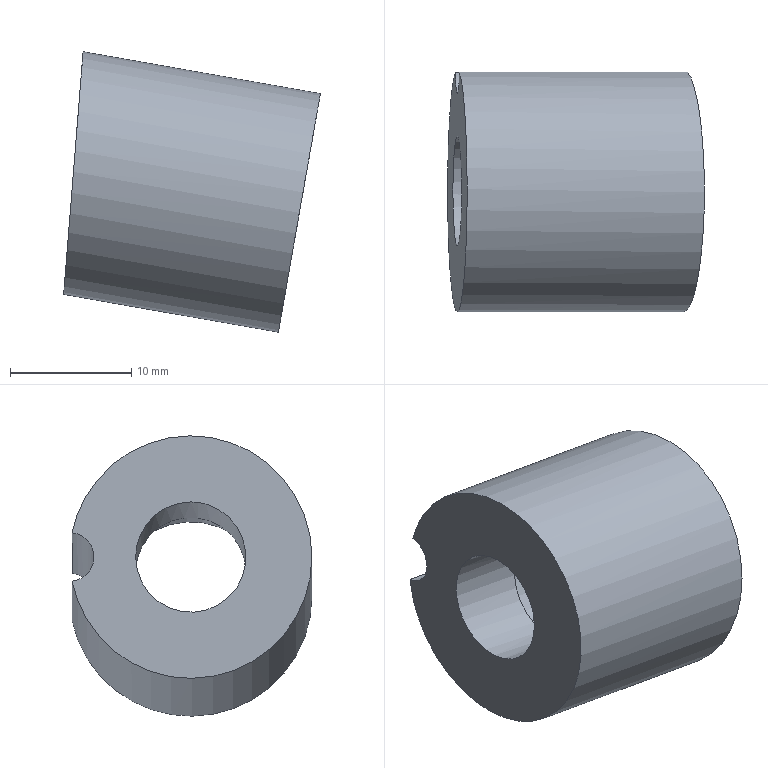Part | NX | features solid 2 | 1 solid | 7 faces | box 21.197 x 19.8 x 23.15 mm | volume 3890 mm3 | cylinder 4 | plane 3 | commonest cylinder face diameters 4 x1 9.1 x1 12.6 x1 20 x1
STEP:
#1=CARTESIAN_POINT('',(-453.088,686.016,-36.598));
#2=VERTEX_POINT('',#1);
#3=CARTESIAN_POINT('',(-434.245,686.016,-39.921));
#4=VERTEX_POINT('',#3);
#5=CARTESIAN_POINT('',(-444.093,686.016,-38.184));
#6=DIRECTION('',(-0.9848,0.,0.1736));
#7=VECTOR('',#6,1000.);
#8=LINE('',#5,#7);
#9=EDGE_CURVE('',#2,#4,#8,.F.);
#10=ORIENTED_EDGE('',*,*,#9,.F.);
#11=CARTESIAN_POINT('',(-453.408,686.016,-40.583));
#12=VERTEX_POINT('',#11);
#13=CARTESIAN_POINT('',(-453.248,676.216,-38.591));
#14=DIRECTION('',(-0.9968,0.,0.08003));
#15=DIRECTION('',(0.08003,0.,0.9968));
#16=AXIS2_PLACEMENT_3D('',#13,#14,#15);
#17=ELLIPSE('',#16,10.045,10.);
#18=EDGE_CURVE('',#2,#12,#17,.F.);
#19=ORIENTED_EDGE('',*,*,#18,.T.);
#20=CARTESIAN_POINT('',(-434.936,686.016,-43.84));
#21=VERTEX_POINT('',#20);
#22=CARTESIAN_POINT('',(-444.784,686.016,-42.104));
#23=DIRECTION('',(-0.9848,0.,0.1736));
#24=VECTOR('',#23,1000.);
#25=LINE('',#22,#24);
#26=EDGE_CURVE('',#21,#12,#25,.T.);
#27=ORIENTED_EDGE('',*,*,#26,.F.);
#28=CARTESIAN_POINT('',(-434.591,676.216,-41.881));
#29=DIRECTION('',(-0.9848,0.,0.1736));
#30=DIRECTION('',(0.,1.,0.));
#31=AXIS2_PLACEMENT_3D('',#28,#29,#30);
#32=CIRCLE('',#31,10.);
#33=EDGE_CURVE('',#21,#4,#32,.T.);
#34=ORIENTED_EDGE('',*,*,#33,.T.);
#35=EDGE_LOOP('',(#10,#19,#27,#34));
#36=FACE_BOUND('',#35,.T.);
#37=CARTESIAN_POINT('',(-434.591,676.216,-41.881));
#38=DIRECTION('',(-0.9848,0.,0.1736));
#39=DIRECTION('',(0.,1.,0.));
#40=AXIS2_PLACEMENT_3D('',#37,#38,#39);
#41=CYLINDRICAL_SURFACE('',#40,10.);
#42=ADVANCED_FACE('',(#36),#41,.T.);
#43=CARTESIAN_POINT('',(-453.248,686.216,-38.591));
#44=DIRECTION('',(-0.9968,0.,0.08003));
#45=DIRECTION('',(0.08003,0.,0.9968));
#46=AXIS2_PLACEMENT_3D('',#43,#44,#45);
#47=ELLIPSE('',#46,2.009,2.);
#48=EDGE_CURVE('',#2,#12,#47,.F.);
#49=ORIENTED_EDGE('',*,*,#48,.F.);
#50=ORIENTED_EDGE('',*,*,#9,.T.);
#51=CARTESIAN_POINT('',(-434.591,686.216,-41.881));
#52=DIRECTION('',(-0.9848,0.,0.1736));
#53=DIRECTION('',(0.,1.,0.));
#54=AXIS2_PLACEMENT_3D('',#51,#52,#53);
#55=CIRCLE('',#54,2.);
#56=EDGE_CURVE('',#21,#4,#55,.T.);
#57=ORIENTED_EDGE('',*,*,#56,.F.);
#58=ORIENTED_EDGE('',*,*,#26,.T.);
#59=EDGE_LOOP('',(#49,#50,#57,#58));
#60=FACE_BOUND('',#59,.T.);
#61=CARTESIAN_POINT('',(-434.591,686.216,-41.881));
#62=DIRECTION('',(-0.9848,0.,0.1736));
#63=DIRECTION('',(0.,1.,0.));
#64=AXIS2_PLACEMENT_3D('',#61,#62,#63);
#65=CYLINDRICAL_SURFACE('',#64,2.);
#66=ADVANCED_FACE('',(#60),#65,.F.);
#67=CARTESIAN_POINT('',(-446.408,680.766,-39.797));
#68=VERTEX_POINT('',#67);
#69=CARTESIAN_POINT('',(-446.408,676.216,-39.797));
#70=DIRECTION('',(-0.9848,0.,0.1736));
#71=DIRECTION('',(0.,1.,0.));
#72=AXIS2_PLACEMENT_3D('',#69,#70,#71);
#73=CIRCLE('',#72,4.55);
#74=EDGE_CURVE('',#68,#68,#73,.T.);
#75=ORIENTED_EDGE('',*,*,#74,.F.);
#76=EDGE_LOOP('',(#75));
#77=FACE_BOUND('',#76,.T.);
#78=CARTESIAN_POINT('',(-452.882,676.216,-34.035));
#79=VERTEX_POINT('',#78);
#80=CARTESIAN_POINT('',(-453.248,676.216,-38.591));
#81=DIRECTION('',(-0.9968,0.,0.08003));
#82=DIRECTION('',(0.08003,0.,0.9968));
#83=AXIS2_PLACEMENT_3D('',#80,#81,#82);
#84=ELLIPSE('',#83,4.57,4.55);
#85=EDGE_CURVE('',#79,#79,#84,.F.);
#86=ORIENTED_EDGE('',*,*,#85,.F.);
#87=EDGE_LOOP('',(#86));
#88=FACE_BOUND('',#87,.T.);
#89=CARTESIAN_POINT('',(-434.591,676.216,-41.881));
#90=DIRECTION('',(-0.9848,0.,0.1736));
#91=DIRECTION('',(0.,1.,0.));
#92=AXIS2_PLACEMENT_3D('',#89,#90,#91);
#93=CYLINDRICAL_SURFACE('',#92,4.55);
#94=ADVANCED_FACE('',(#77,#88),#93,.F.);
#95=CARTESIAN_POINT('',(-434.591,682.516,-41.881));
#96=VERTEX_POINT('',#95);
#97=CARTESIAN_POINT('',(-434.591,676.216,-41.881));
#98=DIRECTION('',(-0.9848,0.,0.1736));
#99=DIRECTION('',(0.,1.,0.));
#100=AXIS2_PLACEMENT_3D('',#97,#98,#99);
#101=CIRCLE('',#100,6.3);
#102=EDGE_CURVE('',#96,#96,#101,.T.);
#103=ORIENTED_EDGE('',*,*,#102,.T.);
#104=EDGE_LOOP('',(#103));
#105=FACE_BOUND('',#104,.T.);
#106=ORIENTED_EDGE('',*,*,#33,.F.);
#107=ORIENTED_EDGE('',*,*,#56,.T.);
#108=EDGE_LOOP('',(#106,#107));
#109=FACE_BOUND('',#108,.T.);
#110=CARTESIAN_POINT('',(-434.591,676.216,-41.881));
#111=DIRECTION('',(-0.9848,0.,0.1736));
#112=DIRECTION('',(0.,1.,0.));
#113=AXIS2_PLACEMENT_3D('',#110,#111,#112);
#114=PLANE('',#113);
#115=ADVANCED_FACE('',(#105,#109),#114,.F.);
#116=ORIENTED_EDGE('',*,*,#102,.F.);
#117=EDGE_LOOP('',(#116));
#118=FACE_BOUND('',#117,.T.);
#119=CARTESIAN_POINT('',(-446.408,682.516,-39.797));
#120=VERTEX_POINT('',#119);
#121=CARTESIAN_POINT('',(-446.408,676.216,-39.797));
#122=DIRECTION('',(-0.9848,0.,0.1736));
#123=DIRECTION('',(0.,1.,0.));
#124=AXIS2_PLACEMENT_3D('',#121,#122,#123);
#125=CIRCLE('',#124,6.3);
#126=EDGE_CURVE('',#120,#120,#125,.T.);
#127=ORIENTED_EDGE('',*,*,#126,.T.);
#128=EDGE_LOOP('',(#127));
#129=FACE_BOUND('',#128,.T.);
#130=CARTESIAN_POINT('',(-434.591,676.216,-41.881));
#131=DIRECTION('',(-0.9848,0.,0.1736));
#132=DIRECTION('',(0.,1.,0.));
#133=AXIS2_PLACEMENT_3D('',#130,#131,#132);
#134=CYLINDRICAL_SURFACE('',#133,6.3);
#135=ADVANCED_FACE('',(#118,#129),#134,.F.);
#136=ORIENTED_EDGE('',*,*,#74,.T.);
#137=EDGE_LOOP('',(#136));
#138=FACE_BOUND('',#137,.T.);
#139=ORIENTED_EDGE('',*,*,#126,.F.);
#140=EDGE_LOOP('',(#139));
#141=FACE_BOUND('',#140,.T.);
#142=CARTESIAN_POINT('',(-446.408,676.216,-39.797));
#143=DIRECTION('',(-0.9848,0.,0.1736));
#144=DIRECTION('',(0.,1.,0.));
#145=AXIS2_PLACEMENT_3D('',#142,#143,#144);
#146=PLANE('',#145);
#147=ADVANCED_FACE('',(#138,#141),#146,.F.);
#148=ORIENTED_EDGE('',*,*,#18,.F.);
#149=ORIENTED_EDGE('',*,*,#48,.T.);
#150=EDGE_LOOP('',(#148,#149));
#151=FACE_BOUND('',#150,.T.);
#152=ORIENTED_EDGE('',*,*,#85,.T.);
#153=EDGE_LOOP('',(#152));
#154=FACE_BOUND('',#153,.T.);
#155=CARTESIAN_POINT('',(-448.537,482.597,20.085));
#156=DIRECTION('',(-0.9968,0.,0.08003));
#157=DIRECTION('',(-0.08003,0.,-0.9968));
#158=AXIS2_PLACEMENT_3D('',#155,#156,#157);
#159=PLANE('',#158);
#160=ADVANCED_FACE('',(#151,#154),#159,.T.);
#161=CLOSED_SHELL('',(#42,#66,#94,#115,#135,#147,#160));
#162=MANIFOLD_SOLID_BREP('',#161);
#163=(LENGTH_UNIT()NAMED_UNIT(*)SI_UNIT(.MILLI.,.METRE.));
#164=UNCERTAINTY_MEASURE_WITH_UNIT(LENGTH_MEASURE(0.00001),#163,'','');
#165=(NAMED_UNIT(*)PLANE_ANGLE_UNIT()SI_UNIT($,.RADIAN.));
#166=(NAMED_UNIT(*)SI_UNIT($,.STERADIAN.)SOLID_ANGLE_UNIT());
#167=(GEOMETRIC_REPRESENTATION_CONTEXT(3)GLOBAL_UNCERTAINTY_ASSIGNED_CONTEXT((#164))GLOBAL_UNIT_ASSIGNED_CONTEXT((#163,#165,#166))REPRESENTATION_CONTEXT('',''));
#168=ADVANCED_BREP_SHAPE_REPRESENTATION('',(#162),#167);